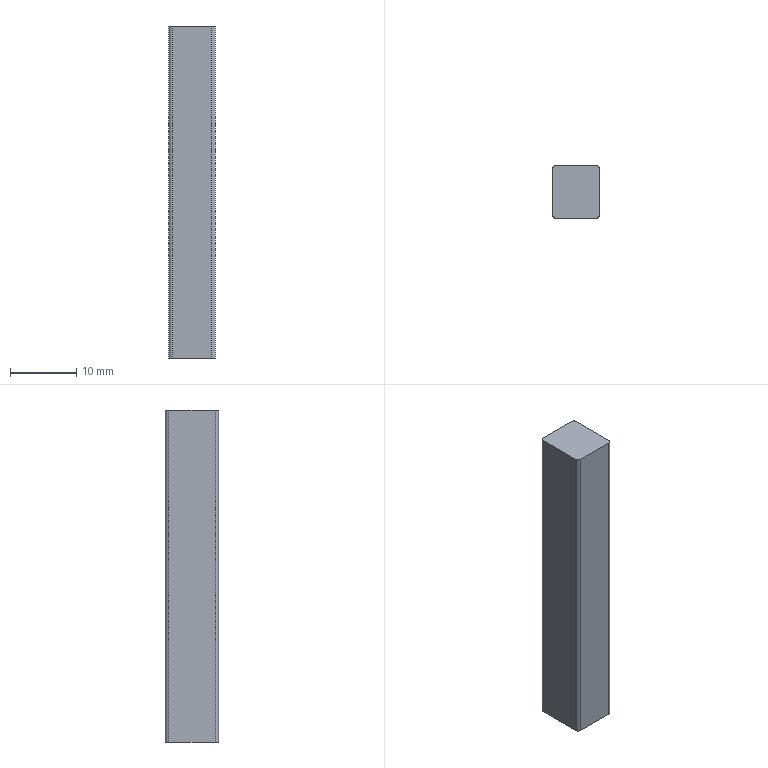Part | NX | features BREP 1 | 1 solid | 10 faces | box 7 x 8 x 50 mm | volume 2789 mm3 | plane 6 | cylinder 4 | commonest cylinder face diameters 1 x4
STEP:
#1=CARTESIAN_POINT('',(-3.,4.,-40.6));
#2=VERTEX_POINT('',#1);
#3=CARTESIAN_POINT('',(-3.5,3.5,-40.6));
#4=VERTEX_POINT('',#3);
#5=CARTESIAN_POINT('',(-3.,3.5,-40.6));
#6=DIRECTION('',(0.,0.,1.));
#7=DIRECTION('',(1.,0.,0.));
#8=AXIS2_PLACEMENT_3D('',#5,#6,#7);
#9=CIRCLE('',#8,0.5);
#10=EDGE_CURVE('',#2,#4,#9,.T.);
#11=ORIENTED_EDGE('',*,*,#10,.F.);
#12=CARTESIAN_POINT('',(-3.,4.,-90.6));
#13=VERTEX_POINT('',#12);
#14=CARTESIAN_POINT('',(-3.,4.,-90.6));
#15=DIRECTION('',(0.,0.,1.));
#16=VECTOR('',#15,1000.);
#17=LINE('',#14,#16);
#18=EDGE_CURVE('',#13,#2,#17,.T.);
#19=ORIENTED_EDGE('',*,*,#18,.F.);
#20=CARTESIAN_POINT('',(-3.5,3.5,-90.6));
#21=VERTEX_POINT('',#20);
#22=CARTESIAN_POINT('',(-3.,3.5,-90.6));
#23=DIRECTION('',(0.,0.,1.));
#24=DIRECTION('',(1.,0.,0.));
#25=AXIS2_PLACEMENT_3D('',#22,#23,#24);
#26=CIRCLE('',#25,0.5);
#27=EDGE_CURVE('',#13,#21,#26,.T.);
#28=ORIENTED_EDGE('',*,*,#27,.T.);
#29=CARTESIAN_POINT('',(-3.5,3.5,-90.6));
#30=DIRECTION('',(0.,0.,1.));
#31=VECTOR('',#30,1000.);
#32=LINE('',#29,#31);
#33=EDGE_CURVE('',#21,#4,#32,.T.);
#34=ORIENTED_EDGE('',*,*,#33,.T.);
#35=EDGE_LOOP('',(#11,#19,#28,#34));
#36=FACE_BOUND('',#35,.T.);
#37=CARTESIAN_POINT('',(-3.,3.5,-90.6));
#38=DIRECTION('',(0.,0.,1.));
#39=DIRECTION('',(-1.,0.,0.));
#40=AXIS2_PLACEMENT_3D('',#37,#38,#39);
#41=CYLINDRICAL_SURFACE('',#40,0.5);
#42=ADVANCED_FACE('',(#36),#41,.T.);
#43=CARTESIAN_POINT('',(-3.5,-3.5,-40.6));
#44=VERTEX_POINT('',#43);
#45=CARTESIAN_POINT('',(-3.5,-3.5,-40.6));
#46=DIRECTION('',(0.,1.,0.));
#47=VECTOR('',#46,1000.);
#48=LINE('',#45,#47);
#49=EDGE_CURVE('',#44,#4,#48,.T.);
#50=ORIENTED_EDGE('',*,*,#49,.T.);
#51=ORIENTED_EDGE('',*,*,#33,.F.);
#52=CARTESIAN_POINT('',(-3.5,-3.5,-90.6));
#53=VERTEX_POINT('',#52);
#54=CARTESIAN_POINT('',(-3.5,-3.5,-90.6));
#55=DIRECTION('',(0.,1.,0.));
#56=VECTOR('',#55,1000.);
#57=LINE('',#54,#56);
#58=EDGE_CURVE('',#53,#21,#57,.T.);
#59=ORIENTED_EDGE('',*,*,#58,.F.);
#60=CARTESIAN_POINT('',(-3.5,-3.5,-90.6));
#61=DIRECTION('',(0.,0.,1.));
#62=VECTOR('',#61,1000.);
#63=LINE('',#60,#62);
#64=EDGE_CURVE('',#53,#44,#63,.T.);
#65=ORIENTED_EDGE('',*,*,#64,.T.);
#66=EDGE_LOOP('',(#50,#51,#59,#65));
#67=FACE_BOUND('',#66,.T.);
#68=CARTESIAN_POINT('',(-3.5,-3.5,-90.6));
#69=DIRECTION('',(1.,0.,0.));
#70=DIRECTION('',(0.,0.,1.));
#71=AXIS2_PLACEMENT_3D('',#68,#69,#70);
#72=PLANE('',#71);
#73=ADVANCED_FACE('',(#67),#72,.F.);
#74=CARTESIAN_POINT('',(-3.,-4.,-40.6));
#75=VERTEX_POINT('',#74);
#76=CARTESIAN_POINT('',(-3.,-3.5,-40.6));
#77=DIRECTION('',(0.,0.,1.));
#78=DIRECTION('',(1.,0.,0.));
#79=AXIS2_PLACEMENT_3D('',#76,#77,#78);
#80=CIRCLE('',#79,0.5);
#81=EDGE_CURVE('',#44,#75,#80,.T.);
#82=ORIENTED_EDGE('',*,*,#81,.F.);
#83=ORIENTED_EDGE('',*,*,#64,.F.);
#84=CARTESIAN_POINT('',(-3.,-4.,-90.6));
#85=VERTEX_POINT('',#84);
#86=CARTESIAN_POINT('',(-3.,-3.5,-90.6));
#87=DIRECTION('',(0.,0.,1.));
#88=DIRECTION('',(1.,0.,0.));
#89=AXIS2_PLACEMENT_3D('',#86,#87,#88);
#90=CIRCLE('',#89,0.5);
#91=EDGE_CURVE('',#53,#85,#90,.T.);
#92=ORIENTED_EDGE('',*,*,#91,.T.);
#93=CARTESIAN_POINT('',(-3.,-4.,-90.6));
#94=DIRECTION('',(0.,0.,1.));
#95=VECTOR('',#94,1000.);
#96=LINE('',#93,#95);
#97=EDGE_CURVE('',#85,#75,#96,.T.);
#98=ORIENTED_EDGE('',*,*,#97,.T.);
#99=EDGE_LOOP('',(#82,#83,#92,#98));
#100=FACE_BOUND('',#99,.T.);
#101=CARTESIAN_POINT('',(-3.,-3.5,-90.6));
#102=DIRECTION('',(0.,0.,1.));
#103=DIRECTION('',(-1.,0.,0.));
#104=AXIS2_PLACEMENT_3D('',#101,#102,#103);
#105=CYLINDRICAL_SURFACE('',#104,0.5);
#106=ADVANCED_FACE('',(#100),#105,.T.);
#107=CARTESIAN_POINT('',(3.,-4.,-40.6));
#108=VERTEX_POINT('',#107);
#109=CARTESIAN_POINT('',(3.,-4.,-40.6));
#110=DIRECTION('',(-1.,0.,0.));
#111=VECTOR('',#110,1000.);
#112=LINE('',#109,#111);
#113=EDGE_CURVE('',#108,#75,#112,.T.);
#114=ORIENTED_EDGE('',*,*,#113,.T.);
#115=ORIENTED_EDGE('',*,*,#97,.F.);
#116=CARTESIAN_POINT('',(3.,-4.,-90.6));
#117=VERTEX_POINT('',#116);
#118=CARTESIAN_POINT('',(3.,-4.,-90.6));
#119=DIRECTION('',(-1.,0.,0.));
#120=VECTOR('',#119,1000.);
#121=LINE('',#118,#120);
#122=EDGE_CURVE('',#117,#85,#121,.T.);
#123=ORIENTED_EDGE('',*,*,#122,.F.);
#124=CARTESIAN_POINT('',(3.,-4.,-90.6));
#125=DIRECTION('',(0.,0.,1.));
#126=VECTOR('',#125,1000.);
#127=LINE('',#124,#126);
#128=EDGE_CURVE('',#117,#108,#127,.T.);
#129=ORIENTED_EDGE('',*,*,#128,.T.);
#130=EDGE_LOOP('',(#114,#115,#123,#129));
#131=FACE_BOUND('',#130,.T.);
#132=CARTESIAN_POINT('',(3.,-4.,-90.6));
#133=DIRECTION('',(0.,1.,0.));
#134=DIRECTION('',(0.,0.,-1.));
#135=AXIS2_PLACEMENT_3D('',#132,#133,#134);
#136=PLANE('',#135);
#137=ADVANCED_FACE('',(#131),#136,.F.);
#138=CARTESIAN_POINT('',(3.5,-3.5,-40.6));
#139=VERTEX_POINT('',#138);
#140=CARTESIAN_POINT('',(3.,-3.5,-40.6));
#141=DIRECTION('',(0.,0.,1.));
#142=DIRECTION('',(1.,0.,0.));
#143=AXIS2_PLACEMENT_3D('',#140,#141,#142);
#144=CIRCLE('',#143,0.5);
#145=EDGE_CURVE('',#108,#139,#144,.T.);
#146=ORIENTED_EDGE('',*,*,#145,.F.);
#147=ORIENTED_EDGE('',*,*,#128,.F.);
#148=CARTESIAN_POINT('',(3.5,-3.5,-90.6));
#149=VERTEX_POINT('',#148);
#150=CARTESIAN_POINT('',(3.,-3.5,-90.6));
#151=DIRECTION('',(0.,0.,1.));
#152=DIRECTION('',(1.,0.,0.));
#153=AXIS2_PLACEMENT_3D('',#150,#151,#152);
#154=CIRCLE('',#153,0.5);
#155=EDGE_CURVE('',#117,#149,#154,.T.);
#156=ORIENTED_EDGE('',*,*,#155,.T.);
#157=CARTESIAN_POINT('',(3.5,-3.5,-90.6));
#158=DIRECTION('',(0.,0.,1.));
#159=VECTOR('',#158,1000.);
#160=LINE('',#157,#159);
#161=EDGE_CURVE('',#149,#139,#160,.T.);
#162=ORIENTED_EDGE('',*,*,#161,.T.);
#163=EDGE_LOOP('',(#146,#147,#156,#162));
#164=FACE_BOUND('',#163,.T.);
#165=CARTESIAN_POINT('',(3.,-3.5,-90.6));
#166=DIRECTION('',(0.,0.,1.));
#167=DIRECTION('',(-1.,0.,0.));
#168=AXIS2_PLACEMENT_3D('',#165,#166,#167);
#169=CYLINDRICAL_SURFACE('',#168,0.5);
#170=ADVANCED_FACE('',(#164),#169,.T.);
#171=CARTESIAN_POINT('',(3.5,3.5,-40.6));
#172=VERTEX_POINT('',#171);
#173=CARTESIAN_POINT('',(3.5,3.5,-40.6));
#174=DIRECTION('',(0.,-1.,0.));
#175=VECTOR('',#174,1000.);
#176=LINE('',#173,#175);
#177=EDGE_CURVE('',#172,#139,#176,.T.);
#178=ORIENTED_EDGE('',*,*,#177,.T.);
#179=ORIENTED_EDGE('',*,*,#161,.F.);
#180=CARTESIAN_POINT('',(3.5,3.5,-90.6));
#181=VERTEX_POINT('',#180);
#182=CARTESIAN_POINT('',(3.5,3.5,-90.6));
#183=DIRECTION('',(0.,-1.,0.));
#184=VECTOR('',#183,1000.);
#185=LINE('',#182,#184);
#186=EDGE_CURVE('',#181,#149,#185,.T.);
#187=ORIENTED_EDGE('',*,*,#186,.F.);
#188=CARTESIAN_POINT('',(3.5,3.5,-90.6));
#189=DIRECTION('',(0.,0.,1.));
#190=VECTOR('',#189,1000.);
#191=LINE('',#188,#190);
#192=EDGE_CURVE('',#181,#172,#191,.T.);
#193=ORIENTED_EDGE('',*,*,#192,.T.);
#194=EDGE_LOOP('',(#178,#179,#187,#193));
#195=FACE_BOUND('',#194,.T.);
#196=CARTESIAN_POINT('',(3.5,3.5,-90.6));
#197=DIRECTION('',(-1.,0.,0.));
#198=DIRECTION('',(0.,0.,-1.));
#199=AXIS2_PLACEMENT_3D('',#196,#197,#198);
#200=PLANE('',#199);
#201=ADVANCED_FACE('',(#195),#200,.F.);
#202=CARTESIAN_POINT('',(3.,4.,-40.6));
#203=VERTEX_POINT('',#202);
#204=CARTESIAN_POINT('',(3.,3.5,-40.6));
#205=DIRECTION('',(0.,0.,1.));
#206=DIRECTION('',(1.,0.,0.));
#207=AXIS2_PLACEMENT_3D('',#204,#205,#206);
#208=CIRCLE('',#207,0.5);
#209=EDGE_CURVE('',#172,#203,#208,.T.);
#210=ORIENTED_EDGE('',*,*,#209,.F.);
#211=ORIENTED_EDGE('',*,*,#192,.F.);
#212=CARTESIAN_POINT('',(3.,4.,-90.6));
#213=VERTEX_POINT('',#212);
#214=CARTESIAN_POINT('',(3.,3.5,-90.6));
#215=DIRECTION('',(0.,0.,1.));
#216=DIRECTION('',(1.,0.,0.));
#217=AXIS2_PLACEMENT_3D('',#214,#215,#216);
#218=CIRCLE('',#217,0.5);
#219=EDGE_CURVE('',#181,#213,#218,.T.);
#220=ORIENTED_EDGE('',*,*,#219,.T.);
#221=CARTESIAN_POINT('',(3.,4.,-90.6));
#222=DIRECTION('',(0.,0.,1.));
#223=VECTOR('',#222,1000.);
#224=LINE('',#221,#223);
#225=EDGE_CURVE('',#213,#203,#224,.T.);
#226=ORIENTED_EDGE('',*,*,#225,.T.);
#227=EDGE_LOOP('',(#210,#211,#220,#226));
#228=FACE_BOUND('',#227,.T.);
#229=CARTESIAN_POINT('',(3.,3.5,-90.6));
#230=DIRECTION('',(0.,0.,1.));
#231=DIRECTION('',(-1.,0.,0.));
#232=AXIS2_PLACEMENT_3D('',#229,#230,#231);
#233=CYLINDRICAL_SURFACE('',#232,0.5);
#234=ADVANCED_FACE('',(#228),#233,.T.);
#235=CARTESIAN_POINT('',(-3.,4.,-40.6));
#236=DIRECTION('',(1.,0.,0.));
#237=VECTOR('',#236,1000.);
#238=LINE('',#235,#237);
#239=EDGE_CURVE('',#2,#203,#238,.T.);
#240=ORIENTED_EDGE('',*,*,#239,.T.);
#241=ORIENTED_EDGE('',*,*,#225,.F.);
#242=CARTESIAN_POINT('',(-3.,4.,-90.6));
#243=DIRECTION('',(1.,0.,0.));
#244=VECTOR('',#243,1000.);
#245=LINE('',#242,#244);
#246=EDGE_CURVE('',#13,#213,#245,.T.);
#247=ORIENTED_EDGE('',*,*,#246,.F.);
#248=ORIENTED_EDGE('',*,*,#18,.T.);
#249=EDGE_LOOP('',(#240,#241,#247,#248));
#250=FACE_BOUND('',#249,.T.);
#251=CARTESIAN_POINT('',(-3.,4.,-90.6));
#252=DIRECTION('',(0.,-1.,0.));
#253=DIRECTION('',(0.,0.,1.));
#254=AXIS2_PLACEMENT_3D('',#251,#252,#253);
#255=PLANE('',#254);
#256=ADVANCED_FACE('',(#250),#255,.F.);
#257=ORIENTED_EDGE('',*,*,#27,.F.);
#258=ORIENTED_EDGE('',*,*,#246,.T.);
#259=ORIENTED_EDGE('',*,*,#219,.F.);
#260=ORIENTED_EDGE('',*,*,#186,.T.);
#261=ORIENTED_EDGE('',*,*,#155,.F.);
#262=ORIENTED_EDGE('',*,*,#122,.T.);
#263=ORIENTED_EDGE('',*,*,#91,.F.);
#264=ORIENTED_EDGE('',*,*,#58,.T.);
#265=EDGE_LOOP('',(#257,#258,#259,#260,#261,#262,#263,#264));
#266=FACE_BOUND('',#265,.T.);
#267=CARTESIAN_POINT('',(-3.,3.5,-90.6));
#268=DIRECTION('',(0.,0.,1.));
#269=DIRECTION('',(-1.,0.,0.));
#270=AXIS2_PLACEMENT_3D('',#267,#268,#269);
#271=PLANE('',#270);
#272=ADVANCED_FACE('',(#266),#271,.F.);
#273=ORIENTED_EDGE('',*,*,#10,.T.);
#274=ORIENTED_EDGE('',*,*,#49,.F.);
#275=ORIENTED_EDGE('',*,*,#81,.T.);
#276=ORIENTED_EDGE('',*,*,#113,.F.);
#277=ORIENTED_EDGE('',*,*,#145,.T.);
#278=ORIENTED_EDGE('',*,*,#177,.F.);
#279=ORIENTED_EDGE('',*,*,#209,.T.);
#280=ORIENTED_EDGE('',*,*,#239,.F.);
#281=EDGE_LOOP('',(#273,#274,#275,#276,#277,#278,#279,#280));
#282=FACE_BOUND('',#281,.T.);
#283=CARTESIAN_POINT('',(-3.,3.5,-40.6));
#284=DIRECTION('',(0.,0.,1.));
#285=DIRECTION('',(-1.,0.,0.));
#286=AXIS2_PLACEMENT_3D('',#283,#284,#285);
#287=PLANE('',#286);
#288=ADVANCED_FACE('',(#282),#287,.T.);
#289=CLOSED_SHELL('',(#42,#73,#106,#137,#170,#201,#234,#256,#272,#288));
#290=MANIFOLD_SOLID_BREP('',#289);
#291=(LENGTH_UNIT()NAMED_UNIT(*)SI_UNIT(.MILLI.,.METRE.));
#292=UNCERTAINTY_MEASURE_WITH_UNIT(LENGTH_MEASURE(0.00001),#291,'','');
#293=(NAMED_UNIT(*)PLANE_ANGLE_UNIT()SI_UNIT($,.RADIAN.));
#294=(NAMED_UNIT(*)SI_UNIT($,.STERADIAN.)SOLID_ANGLE_UNIT());
#295=(GEOMETRIC_REPRESENTATION_CONTEXT(3)GLOBAL_UNCERTAINTY_ASSIGNED_CONTEXT((#292))GLOBAL_UNIT_ASSIGNED_CONTEXT((#291,#293,#294))REPRESENTATION_CONTEXT('',''));
#296=ADVANCED_BREP_SHAPE_REPRESENTATION('',(#290),#295);